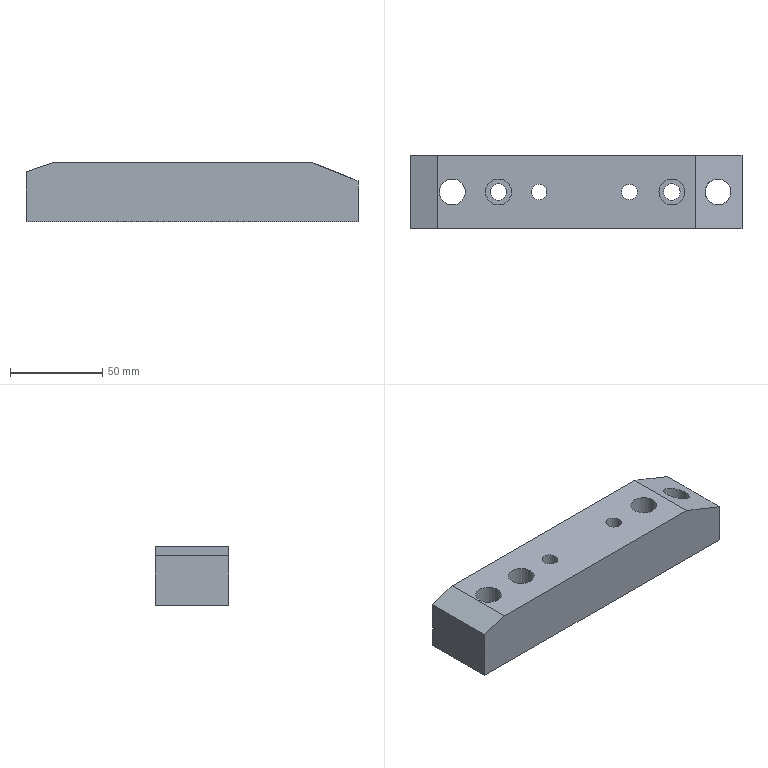Part | STEP file | gslz 2016.10.28-13_id1642_x_t | 1 solid | 22 faces | box 180 x 40 x 32 mm | volume 197761 mm3 | plane 12 | cylinder 10 | commonest cylinder face diameters 14 x4 8.5 x2 9 x2 20 x2